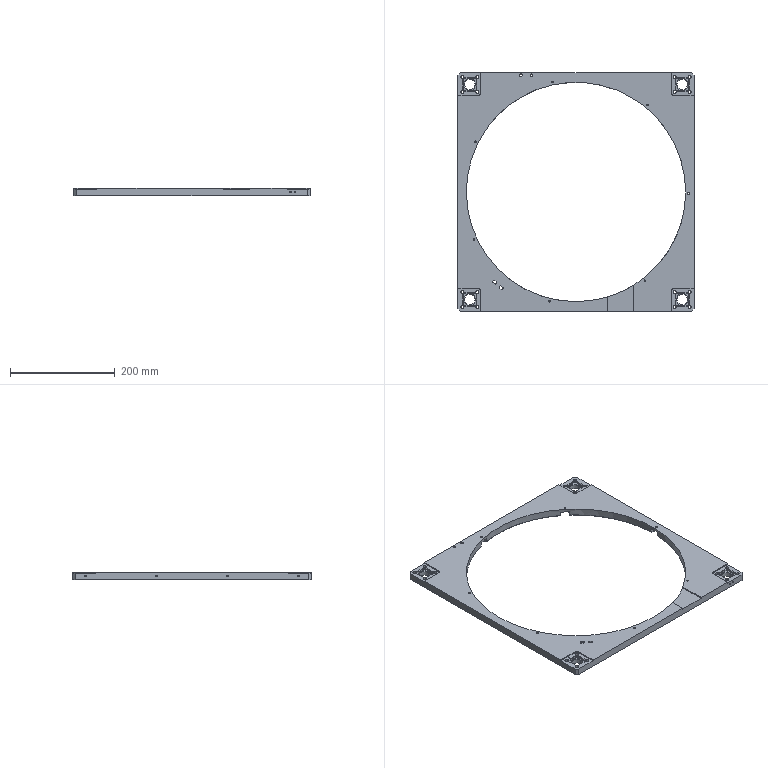Part | NX | features BREP 1 | 1 solid | 333 faces | box 450 x 455 x 15 mm | volume 943273 mm3 | cylinder 165 | plane 102 | cone 66 | commonest cylinder face diameters 5.5 x32 11 x32 3.3 x30 2.5 x20 6 x16 18 x11